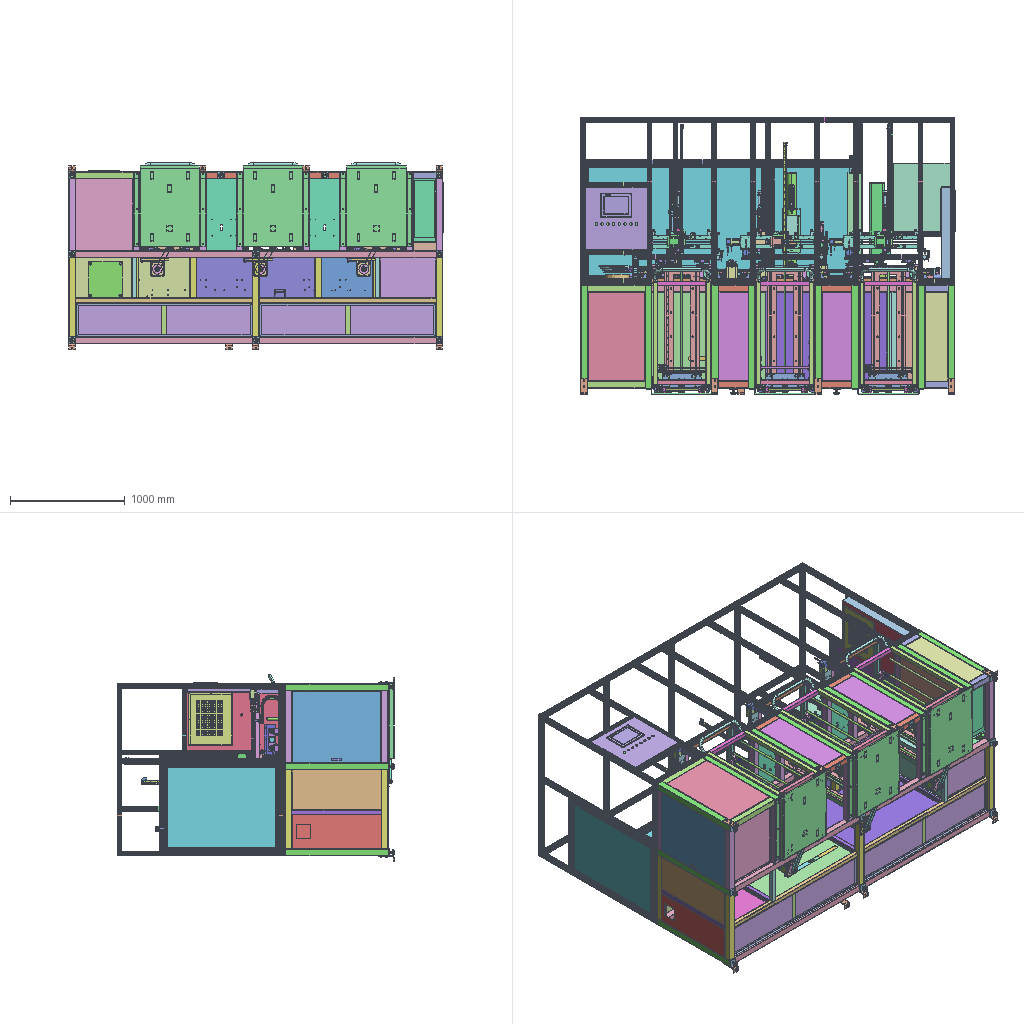Assembly | STEP file | 411 different items | 3950 placed | box 3263 x 2420 x 1630 mm
Parts list (item | name | quantity | parent item | size | volume):
1 | 10 touch screen | x1 | in X77B-00000 | - | -
2 | 12bswbear | x9 | in BSW12_BSW12 | 17.3 x 26.6 x 26.6 mm | 7657 mm3
3 | 12bswcov | x9 | in BSW12_BSW12 | 6.7 x 32.4 x 32.4 mm | 4942 mm3
4 | 12bswnut | x9 | in BSW12_BSW12 | 6.7 x 19 x 19 mm | 1510 mm3
5 | 12bswspa | x9 | in BSW12_BSW12 | 5.5 x 15 x 15 mm | 349.895 mm3
6 | 17 LCD display | x1 | in X77B-00000 | - | -
7 | 350 | x3 | in MGW12C_350_SEBWN14-110 | 24 x 8 x 350 mm | 62774 mm3
8 | 4040-1000 | x1 | in x77-05200 | 40 x 40 x 1000 mm | 703947 mm3
9 | 4040-240 | x1 | in x77-05200 | 40 x 40 x 240 mm | 168947 mm3
10 | 4040-350 | x2 | in x77-05200 | 40 x 40 x 350 mm | 246381 mm3
11 | 4040-450 | x1 | in x77-05200 | 40 x 40 x 450 mm | 316776 mm3
12 | 4040-500 | x1 | in x77-05200 | 40 x 40 x 500 mm | 351974 mm3
13 | 4040-520 | x3 | in x77-05200 | 40 x 40 x 520 mm | 366052 mm3
14 | 4040-540 | x1 | in x77-05200 | 40 x 40 x 540 mm | 380131 mm3
15 | 4040-765 | x6 | in x77-05200 | 40 x 40 x 765 mm | 538519 mm3
16 | 4040-960 | x1 | in x77-05200 | 40 x 40 x 960 mm | 675789 mm3
17 | 40x40-1370 | x6 | in x77-05200 | 40 x 40 x 1370 mm | 964407 mm3
18 | 40x40-1410 | x6 | in x77-05200 | 40 x 40 x 1410 mm | 992565 mm3
19 | 40x40-1420 | x7 | in x77-05200 | 40 x 40 x 1420 mm | 999605 mm3
20 | 40x40-1450 | x4 | in x77-05200 | 40 x 40 x 1450 mm | 1020723 mm3
21 | 40x40-300 | x2 | in x77-05200 | 40 x 40 x 300 mm | 211184 mm3
22 | 40x40-3180 | x3 | in x77-05200 | 40 x 40 x 3180 mm | 2238551 mm3
23 | 40x40-540 | x3 | in x77-05200 | 40 x 40 x 540 mm | 380131 mm3
24 | AS2201_01_F06S_AS2201-01-F06S | x1 | in X77-08200 | 15.5 x 36.4 x 33.9 mm | 6653 mm3
25 | ATPA12L075_A_N16_ATPA12L075-A-N14 | x3 | in X77-07000 | 26 x 45 x 45 mm | 19221 mm3
26 | ATPA12L075_A_P10_ATPA12L075-A-P10 | x3 | in X77-07000 | 26 x 45 x 45 mm | 22986 mm3
27 | A_CXSM20-10-Z73 | x6 | in CXSM20-10-Z73 | 64 x 25.64 x 92 mm | 121716 mm3
28 | BOLT | x24 | in HF-KN43BJ-S100 | 7.112 x 7.112 x 3.81 mm | 129.04 mm3
29 | BS86HB80-04 | x2 | in X77-04000 | 85 x 85 x 128 mm | 650042 mm3
30 | BSW12bsw | x9 | in BSW12_BSW12 | 24 x 43 x 70 mm | 48051 mm3
31 | BUN12bun | x9 | in BUN12_BUN12 | 20 x 43 x 70 mm | 33582 mm3
32 | B_CXSM20-10-Z73 | x6 | in CXSM20-10-Z73 | 62 x 23 x 36 mm | 20357 mm3
33 | Barrel_NP604_B | x2 | in NP604_B_NP604-B | 18.6 x 1.36 x 1.36 mm | 8.939 mm3
34 | Base plate | x4 | in Lamp assembly sw | - | -
35 | CABLE | x6 | in HF-KN43BJ-S100 | 9.906 x 9.906 x 47.625 mm | 1114 mm3
36 | CDP_3_CDP-3 | x6 | in X77-03300 | 12 x 12 x 49.7 mm | 5443 mm3
37 | CD_S03_CD-S03 | x3 | in X77-03300 | 10 x 10 x 34 mm | 2649 mm3
38 | CLGJ50_Rbody | x12 | in CLGJ50_U_CLGJ50-U | 42.667 x 37.625 x 39.322 mm | 4018 mm3
39 | CLGJ50_Rswivel | x12 | in CLGJ50_U_CLGJ50-U | 59 x 9.375 x 47 mm | 14515 mm3
40 | CLGJ50_Uwheel | x12 | in CLGJ50_U_CLGJ50-U | 50 x 50 x 24 mm | 41522 mm3
41 | CLPM16 | x8 | in X77B-02300 | 38 x 50 x 40 mm | 36609 mm3
42 | CM_E032B_CM-E032B | x3 | in X77-03300 | 28 x 53 x 75 mm | 17835 mm3
43 | Cover shell 1 | x56 | in Lamp assembly sw, X77A-09000, X77B-02300, X77B-09000, X77b-01000, x77-09200, x77-09300 | - | -
44 | - | x1 | - | 52 x 52 x 276 mm | 460651 mm3
45 | - | x1 | - | 52 x 52.5 x 226 mm | 470027 mm3
46 | D_BL_D40 | x6 | in CPJC40_BL_10_14_CPJC40-BL-10-14 | 12 x 40 x 36.787 mm | 8300 mm3
47 | FJSM12nut | x10 | in FJSN12_70_FJSN12-70 | 19 x 10 x 21.939 mm | 1964 mm3
48 | FJSN12_70pad | x10 | in FJSN12_70_FJSN12-70 | 50 x 94 x 50 mm | 35453 mm3
49 | - | x10 | in MHZ2_16D_M9N_A_MHZ2-16D-M9N (14.9) | 15.9 x 8 x 21.2 mm | 1340 mm3
50 | - | x10 | in MHZ2_16D_M9N_A_MHZ2-16D-M9N (14.9) | 15.9 x 8 x 21.2 mm | 1340 mm3
51 | - | x12 | in X77-03300 | 22.5 x 25.566 x 1 mm | 158.597 mm3
52 | GB/T 119 4×16 | x10 | in X77-02200, X77-02600, X77-08200, X77b-01000 | 16 x 4 x 4 mm | 200.239 mm3
53 | GB/T 119 5×12 | x2 | in X77b-01000 | 12 x 5 x 5 mm | 170.914 mm3
54 | GB/T 119 5×25 | x1 | in X77b-01000 | 25 x 5 x 5 mm | 485.073 mm3
55 | GB/T 119 6×20 | x6 | in X77B-02000 | 20 x 6 x 6 mm | 558.473 mm3
56 | GB/T 15389 M16×200_M16×200 | x4 | in X77-03000 | 16 x 16 x 200 mm | 34031 mm3
57 | GB/T 276 61804_61804-2Z | x24 | in X77-03300 | 7 x 32 x 32 mm | 2319 mm3
58 | GB/T 5783 M10×70 | x3 | in X77-07000 | 76.4 x 18.475 x 16 mm | 5610 mm3
59 | GB/T 6170 M10 | x10 | in X77-03000, X77-07000, X77B-02000 | 15.424 x 17.77 x 8.4 mm | 1049 mm3
60 | GB/T 6170 M16_M16 | x12 | in X77-03000 | 23.219 x 26.75 x 14.8 mm | 3842 mm3
61 | GB/T 6170 M8 | x83 | in X77-04000, X77-06000, X77-08200, X77-08300, X77b-01000 | 12.482 x 14.38 x 6.8 mm | 562.42 mm3
62 | GB/T 6173-M32×2_(M33) | x1 | in X77b-01000 | 48.06 x 55.37 x 16.5 mm | 18235 mm3
63 | GB/T 77 M3×5_M3×5 | x2 | in X77b-01000 | 5 x 3 x 3 mm | 30.605 mm3
64 | GB/T 77 M8×8_M8×8 | x2 | in X77-08300 | 8 x 8 x 8 mm | 254.883 mm3
65 | GB/T 78 M5×10_M5×10 | x12 | in X77-08200, X77-08300, X77b-01000 | 10 x 5 x 5 mm | 123.644 mm3
66 | GB/T 78 M5×8 | x8 | in X77-08300, X77b-01000 | 8 x 5 x 5 mm | 93.812 mm3
67 | GB/T 808 M20×1 | x3 | in CDM2WB20_100_C76_A_CDM2WB20-100-C76(0) | 26.102 x 30.14 x 3.74 mm | 1028 mm3
68 | GB4040-200 | x1 | in X77b-01000 | 40 x 40 x 170 mm | 64619 mm3
69 | - | x6 | in X77-03000 | 80 x 16 x 16 mm | 7223 mm3
70 | - | x2 | in X77-08300 | 28 x 18 x 18 mm | 4331 mm3
71 | - | x4 | in X77B-00000 | 52 x 18 x 18 mm | 7046 mm3
72 | - | x78 | in X77-02200, X77-02600, X77-04300, X77-08200, X77-08300, X77B-02300, X77b-01000 | 13 x 5.5 x 5.5 mm | 134.591 mm3
73 | - | x7 | in X77-08300, X77b-01000 | 15 x 5.5 x 5.5 mm | 148.728 mm3
74 | - | x1 | in X77b-01000 | 19 x 5.5 x 5.5 mm | 177.003 mm3
75 | - | x26 | in X77-04000, X77-06000, X77-06300 | 23 x 5.5 x 5.5 mm | 205.277 mm3
76 | - | x20 | in X77-04300, X77B-02300 | 28 x 5.5 x 5.5 mm | 240.62 mm3
77 | - | x75 | in X77-03300, X77-04000, X77-04300, X77-06000, X77-06300, X77-08200, X77-08300 | 14 x 7 x 7 mm | 263.094 mm3
78 | - | x663 | in X77-03200g, X77-04000, X77-06000, X77-07000, X77b-01000 | 16 x 7 x 7 mm | 288.227 mm3
79 | - | x156 | in X77-03000, X77-03300, X77-04000, X77-06000, X77-07000, X77A-09000, X77B-02000, X77B-02300, X77B-09000, X77c-09000 | 21 x 8.5 x 8.5 mm | 561.928 mm3
80 | - | x82 | in X77-04000, X77-06000, X77B-02300 | 15 x 8.5 x 8.5 mm | 444.118 mm3
81 | - | x24 | in X77-04000, X77-06000 | 25 x 8.5 x 8.5 mm | 640.468 mm3
82 | - | x40 | in X77-04000, X77-06000, X77-07000, X77B-02300 | 35 x 8.5 x 8.5 mm | 836.817 mm3
83 | - | x30 | in X77-04000, X77-06000 | 45 x 8.5 x 8.5 mm | 1033 mm3
84 | - | x56 | in X77A-09000, X77B-02000, X77B-09000, X77c-09000 | 18 x 10 x 10 mm | 743.186 mm3
85 | - | x110 | in X77-03000, X77-03200g, X77-04000, X77-06000, X77-07000, X77B-02000, X77B-02300 | 22 x 10 x 10 mm | 856.284 mm3
86 | - | x112 | in X77-02600, X77-03200g, X77-03300, X77-04000, X77-06000 | 26 x 10 x 10 mm | 969.381 mm3
87 | - | x15 | in X77-04000, X77-06000 | 36 x 10 x 10 mm | 1252 mm3
88 | - | x12 | in X77-04000, X77-06000 | 46 x 10 x 10 mm | 1535 mm3
89 | - | x6 | in X77-03300 | 20 x 13 x 13 mm | 1535 mm3
90 | - | x62 | in X77-03000 | 24 x 13 x 13 mm | 1736 mm3
91 | - | x202 | in X77-02200, X77-04000, X77-06000, X77-07000, X77-08200, X77-08300, X77B-02000, X77b-01000 | 28 x 13 x 13 mm | 1937 mm3
92 | - | x80 | in X77-03000, X77-07000, X77-08200, X77-08300, X77b-01000 | 33 x 13 x 13 mm | 2189 mm3
93 | - | x36 | in X77-04000, X77-06000 | 38 x 13 x 13 mm | 2440 mm3
94 | - | x12 | in X77-07000 | 43 x 13 x 13 mm | 2691 mm3
95 | - | x9 | in X77-04000, X77-06000, X77-07000 | 48 x 13 x 13 mm | 2943 mm3
96 | - | x12 | in X77-04000, X77-06000 | 68 x 13 x 13 mm | 3948 mm3
97 | - | x12 | in X77-04000, X77-06000 | 78 x 13 x 13 mm | 4451 mm3
98 | - | x8 | in X77-08300, X77b-01000 | 8 x 5.5 x 5.5 mm | 56.004 mm3
99 | HBLFSND8_45_HBLFSND8-45 | x20 | in X77-08200, X77-08300 | 45 x 45 x 35 mm | 24695 mm3
100 | HF-KE23B | x6 | in HF-KN43BJ-S100 | 60 x 60 x 37.084 mm | 33182 mm3
101 | HF-KE23B_BACK | x6 | in HF-KN43BJ-S100 | 61.976 x 147.066 x 38.075 mm | 133952 mm3
102 | HF-KE23B_MID | x6 | in HF-KN43BJ-S100 | 62.024 x 62.024 x 76.204 mm | 244430 mm3
103 | HFC8_4590_Bc | x6 | in HFC8_4590_B_HFC8-4590-B | 90 x 45 x 13 mm | 8335 mm3
104 | HGH15 | x46 | in HGH_15-1050, HGH_15-1170, HGH_15-570, HGH_15-970, HGH_15_210 | 34 x 23.7 x 61.7 mm | 37046 mm3
105 | HGH20H | x9 | in X77B-02000, X77B-02300 | 44 x 25.4 x 92.5 mm | 80377 mm3
106 | HGR15-1050 | x6 | in HGH_15-1050 | 15 x 15 x 1050 mm | 193306 mm3
107 | HGR15-1170 | x3 | in HGH_15-1170 | 15 x 15 x 1170 mm | 215420 mm3
108 | HGR15-210 | x2 | in HGH_15_210 | 15 x 15 x 210 mm | 38506 mm3
109 | HGR15-570 | x6 | in HGH_15-570 | 15 x 15 x 570 mm | 104849 mm3
110 | HGR15-970 | x6 | in HGH_15-970 | 15 x 15 x 970 mm | 178822 mm3
111 | HGR20-2500 | x1 | in X77B-02000 | 20 x 17.5 x 2500 mm | 715425 mm3
112 | - | x48 | in SCCN20_20_SCCN20-10 | 5 x 6 x 6 mm | 115.41 mm3
113 | JA20-8-125 | x3 | in X77-04000, X77-06000 | 21 x 21 x 44 mm | 6882 mm3
114 | JA30_10_125_JA30-10-125 | x5 | in X77-08200, X77-08300, X77B-02000, X77b-01000 | 24 x 24 x 49.5 mm | 10958 mm3
115 | JA40_12_125_JA40-12-125 | x1 | in X77b-01000 | 31 x 31 x 60 mm | 23685 mm3
116 | JA40_14_150_JA40-14-150 | x1 | in X77b-01000 | 31 x 31 x 60 mm | 24083 mm3
117 | LASER HEAD D120I | x1 | in 117 | 180 x 140 x 751 mm | 16335319 mm3
118 | LHFR20_LHTR20 | x24 | in X77A-09000, X77B-09000, X77c-09000 | 42 x 54 x 54 mm | 30800 mm3
119 | LHFS_N12_LHFS-N12 | x12 | in X77-08200, X77-08300, X77b-01000 | 30 x 42 x 42 mm | 10118 mm3
120 | L_CPJC40_10 | x6 | in CPJC40_BL_10_14_CPJC40-BL-10-14 | 39 x 40 x 40 mm | 29913 mm3
121 | Lamp cover | x5 | in Lamp assembly sw, X77-06300 | - | -
122 | LeadWire_NRB604_R | x1 | in NRB604_R_NRB604-R | 7 x 0.63 x 0.63 mm | 2.182 mm3
123 | LeadWire_NRB604_W | x1 | in NRB604_W_NRB604-W | 7 x 0.63 x 0.63 mm | 2.182 mm3
124 | M12x1 sensor | x12 | in X77-04000, X77-06000, X77-07000 | - | -
125 | MFMS16 | x12 | in X77-03200g | 37 x 48 x 48 mm | 21555 mm3
126 | MHZ2_16D | x10 | in MHZ2_16D_M9N_A_MHZ2-16D-M9N (14.9) | 38 x 24 x 57.2 mm | 30555 mm3
127 | Mirror X77-02303 | x10 | in X77-04300, X77B-02300 | - | -
128 | Mirror X77a-01301 | x1 | in X77a-01300 | - | -
129 | OB1530-1000 | x10 | in x77-05500, x77-05600 | 15 x 30 x 1000 mm | 237102 mm3
130 | OB1530-450 | x2 | in x77-05600 | 15 x 30 x 450 mm | 102663 mm3
131 | OB1530-760 | x8 | in x77-05500 | 15 x 30 x 760 mm | 178437 mm3
132 | OB4590-L1 | x2 | in X77-08200, X77b-01000 | 90 x 45 x 400 mm | 511223 mm3
133 | OB4590-L2 | x3 | in X77-08200, X77-08300, X77b-01000 | 90 x 45 x 150 mm | 191709 mm3
134 | OB4590-L3 | x1 | in X77-08300 | 90 x 45 x 1100 mm | 1405865 mm3
135 | OB4590-L4 | x1 | in X77-08300 | 90 x 45 x 140 mm | 178928 mm3
136 | PN_0008 nut | x6 | in SFI R1605B1DFC7 729-831, SFI R1605B1DFC7-989-1071 | - | -
137 | Part 13^X77ZZ-01000 | x2 | in X77ZZ-01000 | - | -
138 | Part 14^X77ZZ-01000 | x1 | in X77ZZ-01000 | - | -
139 | Part 1^csb-00000 | x1 | in csb-00000 | - | -
140 | Part 1^yblx-hl-5030 | x21 | in yblx-hl-5030 | - | -
141 | Part 1^yblx-hl-5030_30 | x3 | in yblx-hl-5030_30 | - | -
142 | Part 2^csb-00000 | x1 | in csb-00000 | - | -
143 | Part 2^yblx-hl-5030 | x21 | in yblx-hl-5030 | - | -
144 | Part 2^yblx-hl-5030_30 | x3 | in yblx-hl-5030_30 | - | -
145 | Part 3^LASER HEAD D120I | x1 | in 117 | - | -
146 | Part 3^yblx-hl-5030 | x21 | in yblx-hl-5030 | - | -
147 | Part 3^yblx-hl-5030_30 | x3 | in yblx-hl-5030_30 | - | -
148 | Part 4^MHZ2_16D_M9N | x20 | in MHZ2_16D_M9N_A_MHZ2-16D-M9N (14.9) | - | -
149 | Part 4^X77ZZ-01000 | x2 | in X77ZZ-01000 | - | -
150 | Part 4^yblx-hl-5030 | x21 | in yblx-hl-5030 | - | -
151 | Part 4^yblx-hl-5030_30 | x3 | in yblx-hl-5030_30 | - | -
152 | Part 5^X77ZZ-01000 | x2 | in X77ZZ-01000 | - | -
153 | Part 5^csb-00000 | x1 | in csb-00000 | - | -
154 | Part 6^csb-00000 | x1 | in csb-00000 | - | -
155 | Part 7^csb-00000 | x1 | in csb-00000 | - | -
156 | Part 9^X77ZZ-01000 | x1 | in X77ZZ-01000 | - | -
157 | R_CPJC40_14 | x6 | in CPJC40_BL_10_14_CPJC40-BL-10-14 | 39 x 40 x 40 mm | 28571 mm3
158 | Receptacle_NRB604 | x2 | in NRB604_R_NRB604-R, NRB604_W_NRB604-W | 23.8 x 1.9 x 1.9 mm | 15.467 mm3
159 | - | x1 | - | 16 x 16 x 205 mm | 38897 mm3
160 | - | x1 | - | 16 x 16 x 138 mm | 25426 mm3
161 | SCCN20_20 | x24 | in SCCN20_20_SCCN20-10 | 20 x 32 x 32 mm | 9528 mm3
162 | SFI1605-4 | x9 | in SFI R1605B1DFC7 559-641, SFI R1605B1DFC7 729-831, SFI R1605B1DFC7-989-1071 | 34 x 49 x 50 mm | 32157 mm3
163 | SHAT25b | x12 | in SHAT25_SHAT25 | 70 x 60 x 24 mm | 48947 mm3
164 | SHBZ12_12_SHBZ12-100 | x8 | in X77-08300, X77b-01000 | 12 x 18 x 18 mm | 1675 mm3
165 | SPCN4_M5_B_SPCN4-M5-B | x20 | in X77-04300, X77B-02300 | 26 x 36.2 x 13.856 mm | 3077 mm3
166 | STANDARD CONTRILLER | x1 | in X77B-00000 | 432 x 156 x 371 mm | 567252 mm3
167 | STHRB16_STHRB16 | x12 | in X77-03200g | 32 x 42 x 42 mm | 11327 mm3
168 | STHSB16_STHSB16 | x8 | in X77-08300, X77b-01000 | 32 x 33 x 33 mm | 9412 mm3
169 | STWN10 | x9 | in BUN12_BUN12 | 1 x 14.1 x 11.82 mm | 51.029 mm3
170 | Shape_NP604_B | x2 | in NP604_B_NP604-B | 13.7 x 1.9 x 1.9 mm | 11.415 mm3
171 | - | x12 | in SHAT25_SHAT25 | 31 x 10 x 10 mm | 1084 mm3
172 | Spring | x2 | in X77a-01300 | - | -
173 | Spring [2] | x14 | in Lamp assembly sw, X77B-02300, X77b-01000 | - | -
174 | TBN225L075 | x3 | in X77-07000 | 19.05 x 39.218 x 264.218 mm | 38535 mm3
175 | TRAT2_4_B_3L1_TRAT2.4-B-3-L1 | x2 | in X77-08300 | 6.2 x 9.5 x 103.6 mm | 2671 mm3
176 | TRAT2_4_B_3L2_TRAT2.4-B-3-L1 | x2 | in X77-08300 | 6.2 x 9.5 x 79 mm | 2037 mm3
177 | Welding machine B-TL-A | x35 | in TA-4923 | - | -
178 | Welding machine B-TL-B | x1 | in TA-4923 | - | -
179 | Welding machine B-TL-C | x1 | in TA-4923 | - | -
180 | X77-01302 | x1 | in X77a-01300 | 210 x 150 x 210 mm | 329352 mm3
181 | X77-02002 | x2 | in X77B-02000 | 54 x 58 x 54 mm | 15867 mm3
182 | X77-02003 | x1 | in X77B-02000 | 16 x 16 x 1981 mm | 394354 mm3
183 | X77-02004 | x1 | in X77B-02000 | 16 x 16 x 6 mm | 735.133 mm3
184 | X77-02101 | x3 | in X77-02100 | 100 x 10 x 90 mm | 86365 mm3
185 | X77-02102 | x3 | in X77-02100 | 100 x 122 x 10 mm | 118906 mm3
186 | X77-02103 | x3 | in X77-02100 | 100 x 40 x 12 mm | 39367 mm3
187 | X77-02104 | x3 | in X77-02100 | 60 x 100 x 10 mm | 36617 mm3
188 | X77-02201a | x6 | in X77-02200 | 44.351 x 93.807 x 11.019 mm | 18832 mm3
189 | X77-02211 | x1 | in X77-02610 | 100 x 9 x 90 mm | 77090 mm3
190 | X77-02211 [2] | x7 | in X77-02210 | 100 x 9 x 90 mm | 77090 mm3
191 | X77-02212a_10 | x1 | in X77-02610 | 48 x 100 x 140 mm | 174759 mm3
192 | X77-02212a_10-2 | x7 | in X77-02210 | 48 x 100 x 140 mm | 174699 mm3
193 | X77-02213 | x1 | in X77-02610 | 50 x 100 x 9 mm | 20503 mm3
194 | X77-02213 [2] | x7 | in X77-02210 | 50 x 100 x 9 mm | 23719 mm3
195 | X77-02301 | x8 | in X77B-02300 | 80 x 110 x 15 mm | 89141 mm3
196 | X77-02302 | x8 | in X77B-02300 | 62 x 35 x 12 mm | 17327 mm3
197 | X77-02303 | x10 | in X77-04300, X77B-02300 | 30 x 24 x 55 mm | 12596 mm3
198 | X77-02601a | x1 | in X77-02600 | 44.351 x 93.807 x 11.019 mm | 17666 mm3
199 | X77-03001 | x1 | in X77-03000 | 1087 x 810 x 12 mm | 10265289 mm3
200 | X77-03002 | x1 | in X77-03000 | 1087 x 810 x 12 mm | 9693894 mm3
201 | X77-03003 | x1 | in X77-03000 | 620 x 690 x 12 mm | 5118080 mm3
202 | X77-03004 | x2 | in X77-03000 | 380 x 690 x 12 mm | 3118641 mm3
203 | X77-03005 | x1 | in X77-03000 | 320 x 690 x 12 mm | 2635862 mm3
204 | X77-03006 | x1 | in X77-03000 | 1087 x 810 x 12 mm | 10436415 mm3
205 | X77-03007 | x1 | in X77-03000 | 488 x 348 x 20 mm | 299031 mm3
206 | X77-03008 | x4 | in X77-03000 | 368 x 778 x 20 mm | 516743 mm3
207 | X77-03008Y | x4 | in X77-03000 | 368 x 778 x 20 mm | 514343 mm3
208 | X77-03009y | x1 | in X77-03000 | 1018 x 778 x 20 mm | 1245859 mm3
209 | X77-03010 | x1 | in X77-03000 | 386 x 778 x 20 mm | 512333 mm3
210 | X77-03011 | x2 | in X77-03000 | 301 x 778 x 20 mm | 385520 mm3
211 | X77-03012 | x2 | in X77-03000 | 1538 x 296.5 x 21.5 mm | 229108 mm3
212 | X77-03013 | x2 | in X77-03000 | 508 x 778 x 20 mm | 661245 mm3
213 | X77-03014 | x1 | in X77-03000 | 371.5 x 778 x 66 mm | 527186 mm3
214 | X77-03015 | x1 | in X77-03000 | 348 x 778 x 20 mm | 465951 mm3
215 | X77-03016 | x1 | in X77-03000 | 1018 x 778 x 20 mm | 1283744 mm3
216 | X77-03017 | x1 | in X77-03000 | 498 x 778 x 20 mm | 649039 mm3
217 | X77-03018 | x2 | in X77-03000 | 626 x 778 x 20 mm | 835340 mm3
218 | X77-03019 | x1 | in X77-03000 | 198 x 778 x 20 mm | 282863 mm3
219 | X77-03020 | x2 | in X77-03000 | 258 x 778 x 20 mm | 356098 mm3
220 | X77-03021 | x1 | in X77-03000 | 198 x 553 x 20 mm | 203981 mm3
221 | X77-03022 | x1 | in X77-03000 | 650 x 778 x 145 mm | 963371 mm3
222 | X77-03023 | x1 | in X77-03000 | 563 x 778 x 689.5 mm | 1566199 mm3
223 | X77-03024 | x1 | in X77-03000 | 498 x 628 x 20 mm | 528951 mm3
224 | X77-03025 | x3 | in X77-03000 | 30 x 40 x 40 mm | 7169 mm3
225 | X77-03026 | x2 | in X77-03000 | 1540 x 300 x 1.5 mm | 693000 mm3
226 | X77-03027 | x1 | in X77-03000 | 290 x 310 x 12 mm | 1071411 mm3
227 | X77-03028 | x6 | in X77-03000 | 40 x 100 x 8 mm | 30315 mm3
228 | X77-03029 | x6 | in X77-03000 | 40 x 40 x 30 mm | 33094 mm3
229 | X77-03030 | x6 | in X77-03000 | 40 x 40 x 8 mm | 9570 mm3
230 | X77-03031 | x8 | in X77-03000 | 50 x 140 x 55 mm | 74451 mm3
231 | X77-03101 | x4 | in X77-03100 | 60 x 60 x 3140 mm | 2123501 mm3
232 | X77-03102 | x12 | in X77-03100 | 60 x 60 x 900 mm | 608647 mm3
233 | X77-03103 | x10 | in X77-03100 | 60 x 60 x 12 mm | 42127 mm3
234 | X77-03104 | x10 | in X77-03100 | 60 x 60 x 690 mm | 466629 mm3
235 | X77-03105 | x16 | in X77-03100 | 60 x 60 x 630 mm | 426053 mm3
236 | X77-03108 | x9 | in X77-03100 | 60 x 60 x 780 mm | 527494 mm3
237 | X77-03109 | x2 | in X77-03100 | 60 x 60 x 200 mm | 135255 mm3
238 | X77-03110 | x4 | in X77-03100 | 60 x 60 x 260 mm | 175831 mm3
239 | X77-03111 | x2 | in X77-03100 | 60 x 60 x 500 mm | 338137 mm3
240 | X77-03113 | x12 | in X77-03100 | 54 x 54 x 8 mm | 23328 mm3
241 | X77-03114 | x2 | in X77-03100 | 40 x 40 x 350 mm | 152696 mm3
242 | X77-03115 | x2 | in X77-03100 | 40 x 40 x 1540 mm | 671862 mm3
243 | X77-03116 | x5 | in X77-03100 | 40 x 40 x 780 mm | 340294 mm3
244 | X77-03201a | x6 | in X77-03200g | 260 x 95 x 10 mm | 236897 mm3
245 | X77-03204g | x6 | in X77-03200g | 35 x 260 x 20 mm | 106557 mm3
246 | X77-03205 | x12 | in X77-03200g | 16 x 16 x 100 mm | 20094 mm3
247 | X77-03211g | x6 | in X77-03210 | 200 x 120 x 9 mm | 156017 mm3
248 | X77-03212 | x6 | in X77-03210 | 60 x 9 x 79 mm | 39895 mm3
249 | X77-03212 [2] | x6 | in X77-03210 | 60 x 9 x 79 mm | 39895 mm3
250 | X77-03213 | x12 | in X77-03210 | 52 x 82.746 x 8 mm | 22201 mm3
251 | X77-03301 | x3 | in X77-03300 | 50 x 35 x 50 mm | 24854 mm3
252 | X77-03302 | x3 | in X77-03300 | 620 x 700 x 53 mm | 3816269 mm3
253 | X77-03303 | x3 | in X77-03300 | 38 x 85 x 50 mm | 50589 mm3
254 | X77-03304 | x12 | in X77-03300 | 26 x 65 x 65 mm | 47550 mm3
255 | X77-03305 | x6 | in X77-03300 | 25 x 25 x 400 mm | 187252 mm3
256 | X77-03306 | x3 | in X77-03300 | 50 x 40 x 8 mm | 14859 mm3
257 | X77-03307 | x12 | in X77-03300 | 25 x 25 x 6 mm | 1060 mm3
258 | X77-04001 | x3 | in X77-04000, X77-06000 | 700 x 110 x 20 mm | 1058356 mm3
259 | X77-04002 | x3 | in X77-04000, X77-06000 | 30 x 30 x 40 mm | 5969 mm3
260 | X77-04003 | x3 | in X77-04000, X77-06000 | 140 x 150 x 16 mm | 308847 mm3
261 | X77-04004 | x3 | in X77-04000, X77-06000 | 50 x 35 x 30 mm | 18530 mm3
262 | X77-04005 | x3 | in X77-04000, X77-06000 | 20 x 20 x 8 mm | 2090 mm3
263 | X77-04006 | x6 | in X77-04000, X77-06000 | 30 x 70 x 32 mm | 63128 mm3
264 | X77-04007 | x3 | in X77-04000, X77-06000 | 50 x 45 x 165 mm | 212521 mm3
265 | X77-04010 | x3 | in X77-04000, X77-06000 | 40.473 x 40.401 x 35 mm | 27750 mm3
266 | X77-04011 | x3 | in X77-04000, X77-06000 | 1170 x 20 x 20 mm | 371955 mm3
267 | X77-04012 | x6 | in X77-04000, X77-06000 | 50 x 75 x 60 mm | 24364 mm3
268 | X77-04013 | x6 | in X77-04000, X77-06000 | 30 x 70 x 20 mm | 39455 mm3
269 | X77-04014 | x3 | in X77-04000, X77-06000 | 105.8 x 150 x 10 mm | 141335 mm3
270 | X77-04015 | x3 | in X77-04000, X77-06000 | 70 x 100 x 90 mm | 60860 mm3
271 | X77-04016 | x3 | in X77-04000, X77-06000 | 81 x 180 x 12 mm | 144400 mm3
272 | X77-04017 | x3 | in X77-04000, X77-06000 | 52 x 90 x 8 mm | 36378 mm3
273 | X77-04018 | x3 | in X77-04000, X77-06000 | 25 x 40 x 40 mm | 5299 mm3
274 | X77-04019 | x3 | in X77-04000, X77-06000 | 25 x 40 x 20 mm | 3509 mm3
275 | X77-04020 | x3 | in X77-04000, X77-06000 | 40 x 55 x 98 mm | 43840 mm3
276 | X77-04021 | x3 | in X77-04000, X77-06000 | 105 x 10 x 80 mm | 83083 mm3
277 | X77-04022 | x3 | in X77-04000, X77-06000 | 60 x 30 x 35 mm | 8293 mm3
278 | X77-04023 | x3 | in X77-04000, X77-06000 | 3 x 54 x 40 mm | 5841 mm3
279 | X77-04101 | x6 | in X77-04100 | 200 x 50 x 12 mm | 116026 mm3
280 | X77-04102 | x6 | in X77-04100 | 12 x 120 x 50 mm | 64489 mm3
281 | X77-04103 | x6 | in X77-04100 | 50 x 87.942 x 10 mm | 26434 mm3
282 | X77-04201 | x3 | in X77-04200 | 40 x 40 x 890 mm | 388035 mm3
283 | X77-04201 [2] | x3 | in X77-04200 | 40 x 40 x 890 mm | 388284 mm3
284 | X77-04202 | x6 | in X77-04200 | 40 x 40 x 520 mm | 226863 mm3
285 | X77-04203 | x12 | in X77-04200 | 40 x 40 x 240 mm | 104706 mm3
286 | X77-04204 | x3 | in X77-04200 | 174 x 10 x 80 mm | 136688 mm3
287 | X77-04205 | x6 | in X77-04200 | 40 x 11 x 970 mm | 388716 mm3
288 | X77-04206 | x12 | in X77-04200 | 65 x 80 x 10 mm | 49455 mm3
289 | X77-04207 | x3 | in X77-04200 | 10 x 76.188 x 80 mm | 48758 mm3
290 | X77-04302 | x2 | in X77-04300 | 50 x 66 x 40 mm | 21765 mm3
291 | X77-04401 | x3 | in X77-04400 | 68 x 68 x 62 mm | 85783 mm3
292 | X77-04402 | x3 | in X77-04400 | 390 x 80 x 10 mm | 310892 mm3
293 | X77-04403 | x6 | in X77-04400 | 150 x 42 x 10 mm | 35959 mm3
294 | X77-05401 | x1 | in x77-05400 | 500 x 600 x 430 mm | 1547522 mm3
295 | X77-05501 | x4 | in x77-05500 | 960 x 720 x 4 mm | 2764800 mm3
296 | X77-05601 | x1 | in x77-05600 | 960 x 410 x 4 mm | 1574400 mm3
297 | X77-06302 | x1 | in X77-06300 | 80 x 80 x 50 mm | 43498 mm3
298 | X77-07001 | x3 | in X77-07000 | 300 x 1050 x 12 mm | 1980727 mm3
299 | X77-07003 | x3 | in X77-07000 | 60 x 55 x 44 mm | 104749 mm3
300 | X77-07004 | x3 | in X77-07000 | 80 x 140 x 120 mm | 115961 mm3
301 | X77-07005 | x3 | in X77-07000 | 65 x 22 x 125 mm | 171490 mm3
302 | X77-07005Z | x3 | in X77-07000 | 65 x 22 x 125 mm | 171718 mm3
303 | X77-07006 | x3 | in X77-07000 | 120 x 80 x 8 mm | 74569 mm3
304 | X77-07007 | x3 | in X77-07000 | 80 x 10 x 200 mm | 147003 mm3
305 | X77-07008 | x3 | in X77-07000 | 80 x 40 x 250 mm | 206681 mm3
306 | X77-07101 | x3 | in X77-07100 | 125 x 8 x 340 mm | 334465 mm3
307 | X77-07102 | x6 | in X77-07100 | 117 x 250.648 x 6 mm | 77736 mm3
308 | X77-07103 | x6 | in X77-07100 | 8 x 80 x 270 mm | 172800 mm3
309 | X77-08202 | x1 | in X77-08200 | 120 x 190 x 12 mm | 260641 mm3
310 | X77-08203 | x2 | in X77-08200 | 12 x 12 x 200 mm | 22584 mm3
311 | X77-08301 | x1 | in X77-08300 | 160 x 320 x 12 mm | 585549 mm3
312 | X77-08303 | x1 | in X77-08300 | 126 x 723 x 245 mm | 1470130 mm3
313 | X77-08304 | x1 | in X77-08300 | 50 x 20 x 37 mm | 13752 mm3
314 | X77-08305 | x1 | in X77-08300 | 41 x 75 x 25 mm | 32721 mm3
315 | X77-08306 | x1 | in X77-08300 | 25 x 67 x 2 mm | 3323 mm3
316 | X77-08307 | x1 | in X77-08300 | 85 x 110 x 65 mm | 33590 mm3
317 | X77-08308 | x1 | in X77-08300 | 90 x 45 x 15 mm | 51606 mm3
318 | X77-08309 | x2 | in X77-08300 | 20 x 20 x 58 mm | 11104 mm3
319 | X77-09001 | x6 | in X77A-09000, X77B-09000, X77c-09000 | 500 x 265 x 12 mm | 1248765 mm3
320 | X77-09002 | x6 | in X77A-09000, X77B-09000, X77c-09000 | 20 x 20 x 640 mm | 189382 mm3
321 | X77-09003 | x20 | in X77A-09000, X77B-09000, X77c-09000 | 20 x 20 x 1030 mm | 322539 mm3
322 | X77-09003h | x4 | in X77A-09000 | 20 x 20 x 900 mm | 281698 mm3
323 | X77-09004 | x16 | in X77B-09000, X77c-09000 | 50 x 50 x 4 mm | 4303 mm3
324 | X77-09101 | x3 | in x77-09100 | 487 x 123.546 x 113.683 mm | 184955 mm3
325 | X77-09102 | x6 | in x77-09100 | 40 x 40 x 420 mm | 183605 mm3
326 | X77-09103 | x6 | in x77-09100 | 40 x 40 x 900 mm | 396510 mm3
327 | X77-09104 | x6 | in x77-09100 | 40 x 40 x 560 mm | 239177 mm3
328 | X77-09105 | x6 | in x77-09100 | 40 x 40 x 100 mm | 48681 mm3
329 | X77-09106 | x3 | in x77-09100 | 40 x 40 x 420 mm | 186089 mm3
330 | X77-09107 | x6 | in x77-09100 | 40 x 40 x 560 mm | 239177 mm3
331 | X77-09108 | x3 | in x77-09100 | 40 x 40 x 420 mm | 185038 mm3
332 | X77-09109 | x12 | in x77-09100 | 47 x 60 x 10 mm | 27415 mm3
333 | X77-09110 | x6 | in x77-09100 | 34 x 34 x 10 mm | 5620 mm3
334 | X77-09211a | x4 | in x77-09200, x77-09300 | 460.001 x 6 x 255 mm | 335353 mm3
335 | X77-09213 | x4 | in x77-09200 | 15 x 42 x 15 mm | 5004 mm3
336 | X77-09313 | x16 | in X77-09400, x77-09300 | 15 x 30 x 15 mm | 3215 mm3
337 | X77-09401 | x1 | in X77-09400 | 276.207 x 471.18 x 6.218 mm | 390241 mm3
338 | X77B-01003 | x4 | in X77-08200, X77-08300 | 8 x 120 x 100 mm | 83628 mm3
339 | X77B-01003a | x2 | in X77b-01000 | 12 x 120 x 100 mm | 118865 mm3
340 | X77B-01004 | x8 | in X77-08300, X77b-01000 | 3 x 22 x 22 mm | 1062 mm3
341 | X77B-01005 | x6 | in X77-08300, X77b-01000 | 15 x 15 x 68 mm | 612.5 mm3
342 | X77B-02004 | x1 | in X77B-02000 | 65.2 x 105 x 12 mm | 67302 mm3
343 | X77ZZ-01001 | x1 | in X77ZZ-01000 | 100 x 11 x 65 mm | 65319 mm3
344 | X77a-01301 | x1 | in X77a-01300 | 328.723 x 61.502 x 320.354 mm | 216130 mm3
345 | X77a-01303 | x1 | in X77a-01300 | 100 x 60 x 100 mm | 441306 mm3
346 | X77b-01001 | x2 | in X77-08300, X77b-01000 | 89.876 x 107.85 x 12.061 mm | 78242 mm3
347 | X77b-01002 | x2 | in X77b-01000 | 17 x 51.049 x 12 mm | 6240 mm3
348 | X77b-01006 | x1 | in X77b-01000 | 160 x 320 x 12 mm | 465416 mm3
349 | X77b-01007 | x1 | in X77b-01000 | 60 x 43.5 x 40 mm | 25586 mm3
350 | X77b-01008 | x8 | in X77-08300, X77b-01000 | 16 x 16 x 165 mm | 25170 mm3
351 | X77b-01009 | x4 | in X77-08300, X77b-01000 | 12 x 12 x 300 mm | 33894 mm3
352 | X77b-01010 | x2 | in X77-08200, X77-08300 | 32 x 100 x 10 mm | 28124 mm3
353 | X77b-01010a | x1 | in X77b-01000 | 32 x 100 x 10 mm | 27866 mm3
354 | X77b-01011 | x2 | in X77-08200, X77b-01000 | 32 x 100 x 4 mm | 12800 mm3
355 | X77b-01012 | x2 | in X77-08300, X77b-01000 | 103.905 x 85.005 x 10 mm | 81895 mm3
356 | X77b-01013 | x1 | in X77b-01000 | 23 x 23 x 10 mm | 2229 mm3
357 | X77b-01014 | x1 | in X77b-01000 | 32 x 42 x 30 mm | 25333 mm3
358 | X77b-01015 | x1 | in X77b-01000 | 22 x 8 x 4 mm | 607.396 mm3
359 | X77b-01016 | x1 | in X77b-01000 | 10 x 4 x 12 mm | 480 mm3
360 | X77b-01017 | x1 | in X77b-01000 | 100 x 40 x 16 mm | 53435 mm3
361 | X77b-01018 | x1 | in X77b-01000 | 50 x 80 x 8 mm | 30756 mm3
362 | X77b-08201 | x1 | in X77-08200 | 44.351 x 93.807 x 40.034 mm | 61790 mm3
363 | YSD3810M-RA | x1 | in X77-06000 | 85 x 85 x 128 mm | 650042 mm3
364 | Y_040B_Y-040B | x3 | in X77-03300 | 38 x 24 x 69 mm | 28298 mm3
365 | Y_P010_Y-P010 | x1 | in X77b-01000 | 13.6 x 10 x 21.5 mm | 1582 mm3
366 | ZH10BS_06_06_ZH10BS-06-06 | x1 | in X77-06300 | 32 x 18 x 63 mm | 30323 mm3
367 | ZPT10UNJ10_B5_A10_N_ZPT10UNJ10-B5-A10 | x2 | in X77-06300 | 14 x 68.5 x 16.166 mm | 4501 mm3
368 | bA_CDQ2B40_40DM_M9N_0_ | x6 | in CDQ2B40_40DM_M9N_A_CDQ2B40-40DM-M9N(0) | 52 x 57 x 79.5 mm | 176566 mm3
369 | b_SECWK14 | x1 | in SECWK14_SECWK14 | 34 x 11 x 50 mm | 8847 mm3
370 | bearingB6000ZZ | x9 | in BUN12_BUN12 | 8 x 26 x 26 mm | 3459 mm3
371 | block_SEBWN14 | x6 | in MGW12C_350_SEBWN14-110 | 40 x 11 x 44.3 mm | 13647 mm3
372 | body_A_CDM2B25_100_C76_0_ | x1 | in CDM2B25_100_C76_A_CDM2B25-100-C76(0) | 30 x 52.6 x 188 mm | 108321 mm3
373 | body_A_CDM2B32_150_C76_0_ | x1 | in CDM2B32_150_C76_A_CDM2B32-150-C76(0) | 35.8 x 59.8 x 240 mm | 197747 mm3
374 | body_A_CDM2B32_275_C76_0_ | x1 | in CDM2B32_275_C76_A_CDM2B32-275-C76(0) | 35.8 x 59.8 x 365 mm | 294811 mm3
375 | body_A_CDM2C40F_75_C76_0_ | x3 | in CDM2C40F_75_C76_A_CDM2C40F-75-C76(0) | 44 x 68 x 229 mm | 272575 mm3
376 | body_A_CDM2WB20_100_C76_0_ | x3 | in CDM2WB20_100_C76_A_CDM2WB20-100-C76(0) | 24 x 47.6 x 188 mm | 67570 mm3
377 | body_A_CDM2WB25_150_C76_0_ | x2 | in CDM2WB25_150_C76_A_CDM2WB25-150-C76(0) | 30 x 52.6 x 238 mm | 124557 mm3
378 | body_A_CDM2WB40_150_C76_0_ | x1 | - | 44 x 68 x 270 mm | 325918 mm3
379 | body_A_CJPB10_10_H4_0_ | x1 | in CJPB10_15_H4_A_CJPB10-10-H4(0) | 19 x 21.939 x 40 mm | 5154 mm3
380 | body_A_CJPS4_10_B_0_ | x1 | in CJPS4_10_B_A_CJPS4-10-B(0) | 10 x 11.547 x 24 mm | 1164 mm3
381 | body_A_CXSM20_40_Z80_0_ | x8 | in CXSM20_40_Z80_A_CXSM20-40-Z80(0) | 64 x 25.64 x 122 mm | 162743 mm3
382 | bsbhb115-06 | x3 | in X77-07000 | 110 x 110 x 146 mm | 1174749 mm3
383 | csb-00001 | x2 | in csb-00000 | 172.5 x 125 x 100 mm | 1165193 mm3
384 | csb-00002 | x1 | in csb-00000 | 84.811 x 974 x 85 mm | 5496286 mm3
385 | csb-00003 | x1 | in csb-00000 | 120 x 11 x 150 mm | 192672 mm3
386 | csb-00004 | x1 | in csb-00000 | 155 x 140 x 165 mm | 928209 mm3
387 | e2e-cr8 | x3 | in X77b-01000 | 4 x 4 x 50 mm | 392.699 mm3
388 | l_SECWK14 | x1 | in SECWK14_SECWK14 | 11 x 11 x 38.5 mm | 1486 mm3
389 | oyu4545-10_HBLFSND8-45 | x8 | in X77b-01000 | 45 x 45 x 43 mm | 29401 mm3
390 | - | x3 | in SFI R1605B1DFC7 559-641 | - | -
391 | - | x3 | in SFI R1605B1DFC7 729-831 | - | -
392 | - | x3 | in SFI R1605B1DFC7-989-1071 | - | -
393 | rA_CDQ2B40_40DM_M9N_0_ | x6 | in CDQ2B40_40DM_M9N_A_CDQ2B40-40DM-M9N(0) | 16 x 16 x 69.5 mm | 12766 mm3
394 | rod_A_CDM2B25_100_C76_0_ | x1 | in CDM2B25_100_C76_A_CDM2B25-100-C76(0) | 10 x 10 x 133 mm | 10311 mm3
395 | rod_A_CDM2B32_150_C76_0_ | x1 | in CDM2B32_150_C76_A_CDM2B32-150-C76(0) | 12 x 12 x 183 mm | 19693 mm3
396 | rod_A_CDM2B32_275_C76_0_ | x1 | in CDM2B32_275_C76_A_CDM2B32-275-C76(0) | 12 x 12 x 308 mm | 33830 mm3
397 | rod_A_CDM2C40F_75_C76_0_ | x3 | in CDM2C40F_75_C76_A_CDM2C40F-75-C76(0) | 14 x 14 x 110 mm | 16659 mm3
398 | rod_A_CDM2WB20_100_C76_0_ | x3 | in CDM2WB20_100_C76_A_CDM2WB20-100-C76(0) | 8 x 8 x 344 mm | 17104 mm3
399 | rod_A_CDM2WB25_150_C76_0_ | x2 | in CDM2WB25_150_C76_A_CDM2WB25-150-C76(0) | 10 x 10 x 452 mm | 35231 mm3
400 | rod_A_CDM2WB40_150_C76_0_ | x1 | - | 14 x 14 x 488 mm | 74574 mm3
401 | rod_A_CJPB10_15_H4_0_ | x1 | in CJPB10_15_H4_A_CJPB10-10-H4(0) | 5 x 5 x 23 mm | 444.797 mm3
402 | rod_A_CJPS4_10_B_0_ | x1 | in CJPS4_10_B_A_CJPS4-10-B(0) | 2 x 2 x 18.5 mm | 58.039 mm3
403 | rod_A_CXSM20_40_Z80_0_ | x8 | in CXSM20_40_Z80_A_CXSM20-40-Z80(0) | 62 x 23 x 66 mm | 24938 mm3
404 | x77-05101 | x1 | in x77-05100 | 540 x 553 x 71.5 mm | 640844 mm3
405 | x77-05102 | x1 | in x77-05100 | 535 x 548 x 1.5 mm | 423444 mm3
406 | x77-05301 | x1 | in x77-05300 | 540 x 803 x 120 mm | 1120219 mm3
407 | x77-05302 | x1 | in x77-05300 | 464 x 385 x 1.5 mm | 245190 mm3
408 | x77-05303 | x1 | in x77-05300 | 502 x 365 x 15 mm | 206076 mm3
409 | x77-05402 | x1 | in x77-05400 | 465.4 x 565.4 x 15 mm | 115350 mm3
410 | x77-05403 | x1 | in x77-05400 | 411 x 515 x 3 mm | 634995 mm3
411 | yh610h | x1 | in X77-03000 | 180 x 430 x 490 mm | 672024 mm3